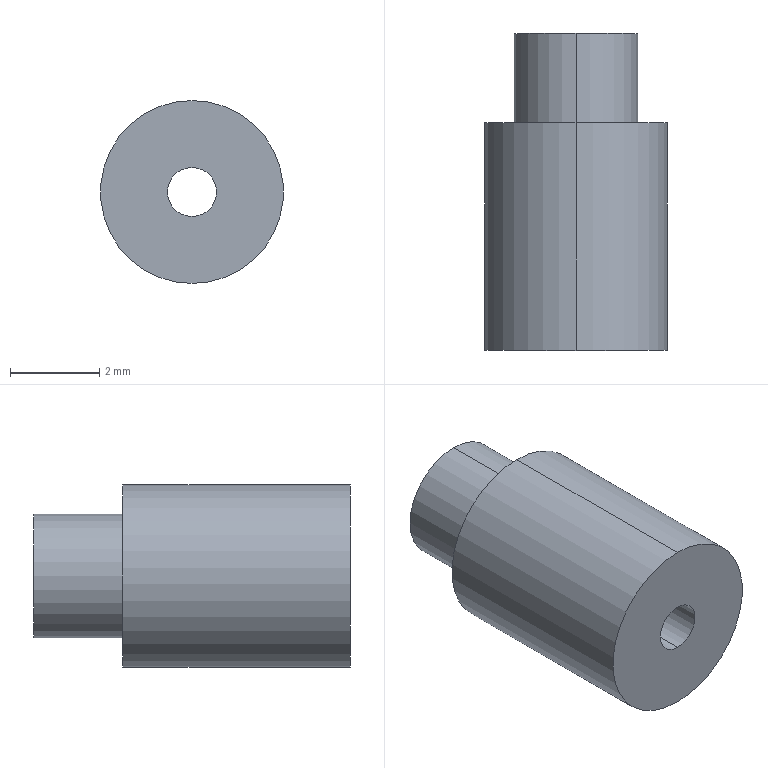Part | SolidWorks | features Revolution 1 | 1 solid | 9 faces | box 4.1 x 7.1 x 4.1 mm | volume 72.551 mm3 | cylinder 6 | plane 3 | commonest cylinder face diameters 1.1 x2 2.76 x2 4.1 x2
STEP:
#1=CARTESIAN_POINT('',(0.,5.6,0.55));
#2=VERTEX_POINT('',#1);
#3=CARTESIAN_POINT('',(0.,5.6,-0.55));
#4=VERTEX_POINT('',#3);
#5=CARTESIAN_POINT('',(0.,5.6,0.));
#6=DIRECTION('',(0.,-1.,0.));
#7=DIRECTION('',(0.,0.,-1.));
#8=AXIS2_PLACEMENT_3D('',#5,#6,#7);
#9=CIRCLE('',#8,0.55);
#10=EDGE_CURVE('',#2,#4,#9,.T.);
#11=ORIENTED_EDGE('',*,*,#10,.F.);
#12=CARTESIAN_POINT('',(0.,-1.5,0.55));
#13=VERTEX_POINT('',#12);
#14=CARTESIAN_POINT('',(0.,-0.7316,0.55));
#15=DIRECTION('',(0.,-1.,0.));
#16=VECTOR('',#15,1000.);
#17=LINE('',#14,#16);
#18=EDGE_CURVE('',#2,#13,#17,.T.);
#19=ORIENTED_EDGE('',*,*,#18,.T.);
#20=CARTESIAN_POINT('',(0.,-1.5,-0.55));
#21=VERTEX_POINT('',#20);
#22=CARTESIAN_POINT('',(0.,-1.5,0.));
#23=DIRECTION('',(0.,-1.,0.));
#24=DIRECTION('',(0.,0.,-1.));
#25=AXIS2_PLACEMENT_3D('',#22,#23,#24);
#26=CIRCLE('',#25,0.55);
#27=EDGE_CURVE('',#13,#21,#26,.T.);
#28=ORIENTED_EDGE('',*,*,#27,.T.);
#29=CARTESIAN_POINT('',(0.,-0.7316,-0.55));
#30=DIRECTION('',(0.,-1.,0.));
#31=VECTOR('',#30,1000.);
#32=LINE('',#29,#31);
#33=EDGE_CURVE('',#4,#21,#32,.T.);
#34=ORIENTED_EDGE('',*,*,#33,.F.);
#35=EDGE_LOOP('',(#11,#19,#28,#34));
#36=FACE_OUTER_BOUND('',#35,.T.);
#37=CARTESIAN_POINT('',(0.,-0.7316,0.));
#38=DIRECTION('',(0.,-1.,0.));
#39=DIRECTION('',(0.,0.,-1.));
#40=AXIS2_PLACEMENT_3D('',#37,#38,#39);
#41=CYLINDRICAL_SURFACE('',#40,0.55);
#42=ADVANCED_FACE('',(#36),#41,.F.);
#43=CARTESIAN_POINT('',(0.,5.6,-1.38));
#44=VERTEX_POINT('',#43);
#45=CARTESIAN_POINT('',(0.,5.6,1.38));
#46=VERTEX_POINT('',#45);
#47=CARTESIAN_POINT('',(0.,5.6,0.));
#48=DIRECTION('',(0.,-1.,0.));
#49=DIRECTION('',(0.,0.,-1.));
#50=AXIS2_PLACEMENT_3D('',#47,#48,#49);
#51=CIRCLE('',#50,1.38);
#52=EDGE_CURVE('',#44,#46,#51,.T.);
#53=ORIENTED_EDGE('',*,*,#52,.T.);
#54=CARTESIAN_POINT('',(0.,3.6,1.38));
#55=VERTEX_POINT('',#54);
#56=CARTESIAN_POINT('',(0.,-0.7316,1.38));
#57=DIRECTION('',(0.,-1.,0.));
#58=VECTOR('',#57,1000.);
#59=LINE('',#56,#58);
#60=EDGE_CURVE('',#46,#55,#59,.T.);
#61=ORIENTED_EDGE('',*,*,#60,.T.);
#62=CARTESIAN_POINT('',(0.,3.6,-1.38));
#63=VERTEX_POINT('',#62);
#64=CARTESIAN_POINT('',(0.,3.6,0.));
#65=DIRECTION('',(0.,-1.,0.));
#66=DIRECTION('',(0.,0.,-1.));
#67=AXIS2_PLACEMENT_3D('',#64,#65,#66);
#68=CIRCLE('',#67,1.38);
#69=EDGE_CURVE('',#63,#55,#68,.T.);
#70=ORIENTED_EDGE('',*,*,#69,.F.);
#71=CARTESIAN_POINT('',(0.,-0.7316,-1.38));
#72=DIRECTION('',(0.,-1.,0.));
#73=VECTOR('',#72,1000.);
#74=LINE('',#71,#73);
#75=EDGE_CURVE('',#44,#63,#74,.T.);
#76=ORIENTED_EDGE('',*,*,#75,.F.);
#77=EDGE_LOOP('',(#53,#61,#70,#76));
#78=FACE_OUTER_BOUND('',#77,.T.);
#79=CARTESIAN_POINT('',(0.,-0.7316,0.));
#80=DIRECTION('',(0.,-1.,0.));
#81=DIRECTION('',(0.,0.,-1.));
#82=AXIS2_PLACEMENT_3D('',#79,#80,#81);
#83=CYLINDRICAL_SURFACE('',#82,1.38);
#84=ADVANCED_FACE('',(#78),#83,.T.);
#85=CARTESIAN_POINT('',(0.,3.6,-2.05));
#86=VERTEX_POINT('',#85);
#87=CARTESIAN_POINT('',(0.,3.6,2.05));
#88=VERTEX_POINT('',#87);
#89=CARTESIAN_POINT('',(0.,3.6,0.));
#90=DIRECTION('',(0.,-1.,0.));
#91=DIRECTION('',(0.,0.,-1.));
#92=AXIS2_PLACEMENT_3D('',#89,#90,#91);
#93=CIRCLE('',#92,2.05);
#94=EDGE_CURVE('',#86,#88,#93,.T.);
#95=ORIENTED_EDGE('',*,*,#94,.T.);
#96=CARTESIAN_POINT('',(0.,-1.5,2.05));
#97=VERTEX_POINT('',#96);
#98=CARTESIAN_POINT('',(0.,-0.7316,2.05));
#99=DIRECTION('',(0.,-1.,0.));
#100=VECTOR('',#99,1000.);
#101=LINE('',#98,#100);
#102=EDGE_CURVE('',#88,#97,#101,.T.);
#103=ORIENTED_EDGE('',*,*,#102,.T.);
#104=CARTESIAN_POINT('',(0.,-1.5,-2.05));
#105=VERTEX_POINT('',#104);
#106=CARTESIAN_POINT('',(0.,-1.5,0.));
#107=DIRECTION('',(0.,-1.,0.));
#108=DIRECTION('',(0.,0.,-1.));
#109=AXIS2_PLACEMENT_3D('',#106,#107,#108);
#110=CIRCLE('',#109,2.05);
#111=EDGE_CURVE('',#105,#97,#110,.T.);
#112=ORIENTED_EDGE('',*,*,#111,.F.);
#113=CARTESIAN_POINT('',(0.,-0.7316,-2.05));
#114=DIRECTION('',(0.,-1.,0.));
#115=VECTOR('',#114,1000.);
#116=LINE('',#113,#115);
#117=EDGE_CURVE('',#86,#105,#116,.T.);
#118=ORIENTED_EDGE('',*,*,#117,.F.);
#119=EDGE_LOOP('',(#95,#103,#112,#118));
#120=FACE_OUTER_BOUND('',#119,.T.);
#121=CARTESIAN_POINT('',(0.,-0.7316,0.));
#122=DIRECTION('',(0.,-1.,0.));
#123=DIRECTION('',(0.,0.,-1.));
#124=AXIS2_PLACEMENT_3D('',#121,#122,#123);
#125=CYLINDRICAL_SURFACE('',#124,2.05);
#126=ADVANCED_FACE('',(#120),#125,.T.);
#127=ORIENTED_EDGE('',*,*,#102,.F.);
#128=CARTESIAN_POINT('',(0.,3.6,0.));
#129=DIRECTION('',(0.,-1.,0.));
#130=DIRECTION('',(0.,0.,-1.));
#131=AXIS2_PLACEMENT_3D('',#128,#129,#130);
#132=CIRCLE('',#131,2.05);
#133=EDGE_CURVE('',#88,#86,#132,.T.);
#134=ORIENTED_EDGE('',*,*,#133,.T.);
#135=ORIENTED_EDGE('',*,*,#117,.T.);
#136=CARTESIAN_POINT('',(0.,-1.5,0.));
#137=DIRECTION('',(0.,-1.,0.));
#138=DIRECTION('',(0.,0.,-1.));
#139=AXIS2_PLACEMENT_3D('',#136,#137,#138);
#140=CIRCLE('',#139,2.05);
#141=EDGE_CURVE('',#97,#105,#140,.T.);
#142=ORIENTED_EDGE('',*,*,#141,.F.);
#143=EDGE_LOOP('',(#127,#134,#135,#142));
#144=FACE_OUTER_BOUND('',#143,.T.);
#145=CARTESIAN_POINT('',(0.,-0.7316,0.));
#146=DIRECTION('',(0.,-1.,0.));
#147=DIRECTION('',(0.,0.,-1.));
#148=AXIS2_PLACEMENT_3D('',#145,#146,#147);
#149=CYLINDRICAL_SURFACE('',#148,2.05);
#150=ADVANCED_FACE('',(#144),#149,.T.);
#151=ORIENTED_EDGE('',*,*,#94,.F.);
#152=ORIENTED_EDGE('',*,*,#133,.F.);
#153=EDGE_LOOP('',(#151,#152));
#154=FACE_OUTER_BOUND('',#153,.T.);
#155=ORIENTED_EDGE('',*,*,#69,.T.);
#156=CARTESIAN_POINT('',(0.,3.6,0.));
#157=DIRECTION('',(0.,-1.,0.));
#158=DIRECTION('',(0.,0.,-1.));
#159=AXIS2_PLACEMENT_3D('',#156,#157,#158);
#160=CIRCLE('',#159,1.38);
#161=EDGE_CURVE('',#55,#63,#160,.T.);
#162=ORIENTED_EDGE('',*,*,#161,.T.);
#163=EDGE_LOOP('',(#155,#162));
#164=FACE_BOUND('',#163,.T.);
#165=CARTESIAN_POINT('',(-2.05,3.6,0.));
#166=DIRECTION('',(0.,-1.,0.));
#167=DIRECTION('',(0.,0.,-1.));
#168=AXIS2_PLACEMENT_3D('',#165,#166,#167);
#169=PLANE('',#168);
#170=ADVANCED_FACE('',(#154,#164),#169,.F.);
#171=ORIENTED_EDGE('',*,*,#60,.F.);
#172=CARTESIAN_POINT('',(0.,5.6,0.));
#173=DIRECTION('',(0.,-1.,0.));
#174=DIRECTION('',(0.,0.,-1.));
#175=AXIS2_PLACEMENT_3D('',#172,#173,#174);
#176=CIRCLE('',#175,1.38);
#177=EDGE_CURVE('',#46,#44,#176,.T.);
#178=ORIENTED_EDGE('',*,*,#177,.T.);
#179=ORIENTED_EDGE('',*,*,#75,.T.);
#180=ORIENTED_EDGE('',*,*,#161,.F.);
#181=EDGE_LOOP('',(#171,#178,#179,#180));
#182=FACE_OUTER_BOUND('',#181,.T.);
#183=CARTESIAN_POINT('',(0.,-0.7316,0.));
#184=DIRECTION('',(0.,-1.,0.));
#185=DIRECTION('',(0.,0.,-1.));
#186=AXIS2_PLACEMENT_3D('',#183,#184,#185);
#187=CYLINDRICAL_SURFACE('',#186,1.38);
#188=ADVANCED_FACE('',(#182),#187,.T.);
#189=ORIENTED_EDGE('',*,*,#52,.F.);
#190=ORIENTED_EDGE('',*,*,#177,.F.);
#191=EDGE_LOOP('',(#189,#190));
#192=FACE_OUTER_BOUND('',#191,.T.);
#193=CARTESIAN_POINT('',(0.,5.6,0.));
#194=DIRECTION('',(0.,-1.,0.));
#195=DIRECTION('',(0.,0.,-1.));
#196=AXIS2_PLACEMENT_3D('',#193,#194,#195);
#197=CIRCLE('',#196,0.55);
#198=EDGE_CURVE('',#4,#2,#197,.T.);
#199=ORIENTED_EDGE('',*,*,#198,.T.);
#200=ORIENTED_EDGE('',*,*,#10,.T.);
#201=EDGE_LOOP('',(#199,#200));
#202=FACE_BOUND('',#201,.T.);
#203=CARTESIAN_POINT('',(-1.38,5.6,0.));
#204=DIRECTION('',(0.,-1.,0.));
#205=DIRECTION('',(0.,0.,-1.));
#206=AXIS2_PLACEMENT_3D('',#203,#204,#205);
#207=PLANE('',#206);
#208=ADVANCED_FACE('',(#192,#202),#207,.F.);
#209=ORIENTED_EDGE('',*,*,#18,.F.);
#210=ORIENTED_EDGE('',*,*,#198,.F.);
#211=ORIENTED_EDGE('',*,*,#33,.T.);
#212=CARTESIAN_POINT('',(0.,-1.5,0.));
#213=DIRECTION('',(0.,-1.,0.));
#214=DIRECTION('',(0.,0.,-1.));
#215=AXIS2_PLACEMENT_3D('',#212,#213,#214);
#216=CIRCLE('',#215,0.55);
#217=EDGE_CURVE('',#21,#13,#216,.T.);
#218=ORIENTED_EDGE('',*,*,#217,.T.);
#219=EDGE_LOOP('',(#209,#210,#211,#218));
#220=FACE_OUTER_BOUND('',#219,.T.);
#221=CARTESIAN_POINT('',(0.,-0.7316,0.));
#222=DIRECTION('',(0.,-1.,0.));
#223=DIRECTION('',(0.,0.,-1.));
#224=AXIS2_PLACEMENT_3D('',#221,#222,#223);
#225=CYLINDRICAL_SURFACE('',#224,0.55);
#226=ADVANCED_FACE('',(#220),#225,.F.);
#227=ORIENTED_EDGE('',*,*,#217,.F.);
#228=ORIENTED_EDGE('',*,*,#27,.F.);
#229=EDGE_LOOP('',(#227,#228));
#230=FACE_BOUND('',#229,.T.);
#231=ORIENTED_EDGE('',*,*,#111,.T.);
#232=ORIENTED_EDGE('',*,*,#141,.T.);
#233=EDGE_LOOP('',(#231,#232));
#234=FACE_OUTER_BOUND('',#233,.T.);
#235=CARTESIAN_POINT('',(-0.55,-1.5,0.));
#236=DIRECTION('',(0.,1.,0.));
#237=DIRECTION('',(0.,0.,1.));
#238=AXIS2_PLACEMENT_3D('',#235,#236,#237);
#239=PLANE('',#238);
#240=ADVANCED_FACE('',(#230,#234),#239,.F.);
#241=CLOSED_SHELL('',(#42,#84,#126,#150,#170,#188,#208,#226,#240));
#242=MANIFOLD_SOLID_BREP('',#241);
#243=CARTESIAN_POINT('',(0.,0.,0.));
#244=DIRECTION('',(0.,0.,1.));
#245=DIRECTION('',(1.,0.,0.));
#246=AXIS2_PLACEMENT_3D('',#243,#244,#245);
#247=(LENGTH_UNIT()NAMED_UNIT(*)SI_UNIT(.MILLI.,.METRE.));
#248=UNCERTAINTY_MEASURE_WITH_UNIT(LENGTH_MEASURE(0.00001),#247,'','');
#249=(NAMED_UNIT(*)PLANE_ANGLE_UNIT()SI_UNIT($,.RADIAN.));
#250=(NAMED_UNIT(*)SI_UNIT($,.STERADIAN.)SOLID_ANGLE_UNIT());
#251=(GEOMETRIC_REPRESENTATION_CONTEXT(3)GLOBAL_UNCERTAINTY_ASSIGNED_CONTEXT((#248))GLOBAL_UNIT_ASSIGNED_CONTEXT((#247,#249,#250))REPRESENTATION_CONTEXT('',''));
#252=ADVANCED_BREP_SHAPE_REPRESENTATION('',(#242,#246),#251);